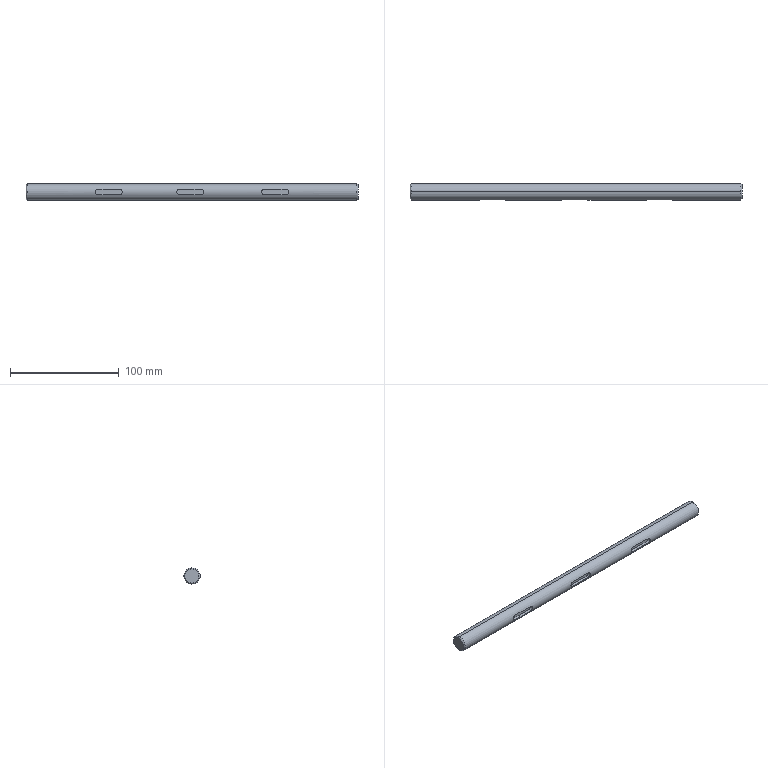Part | STEP file | 0228_205_Shaft | 1 solid | 23 faces | box 305 x 15 x 15 mm | volume 52825 mm3 | plane 11 | cylinder 8 | cone 4 | commonest cylinder face diameters 5 x6 15 x2